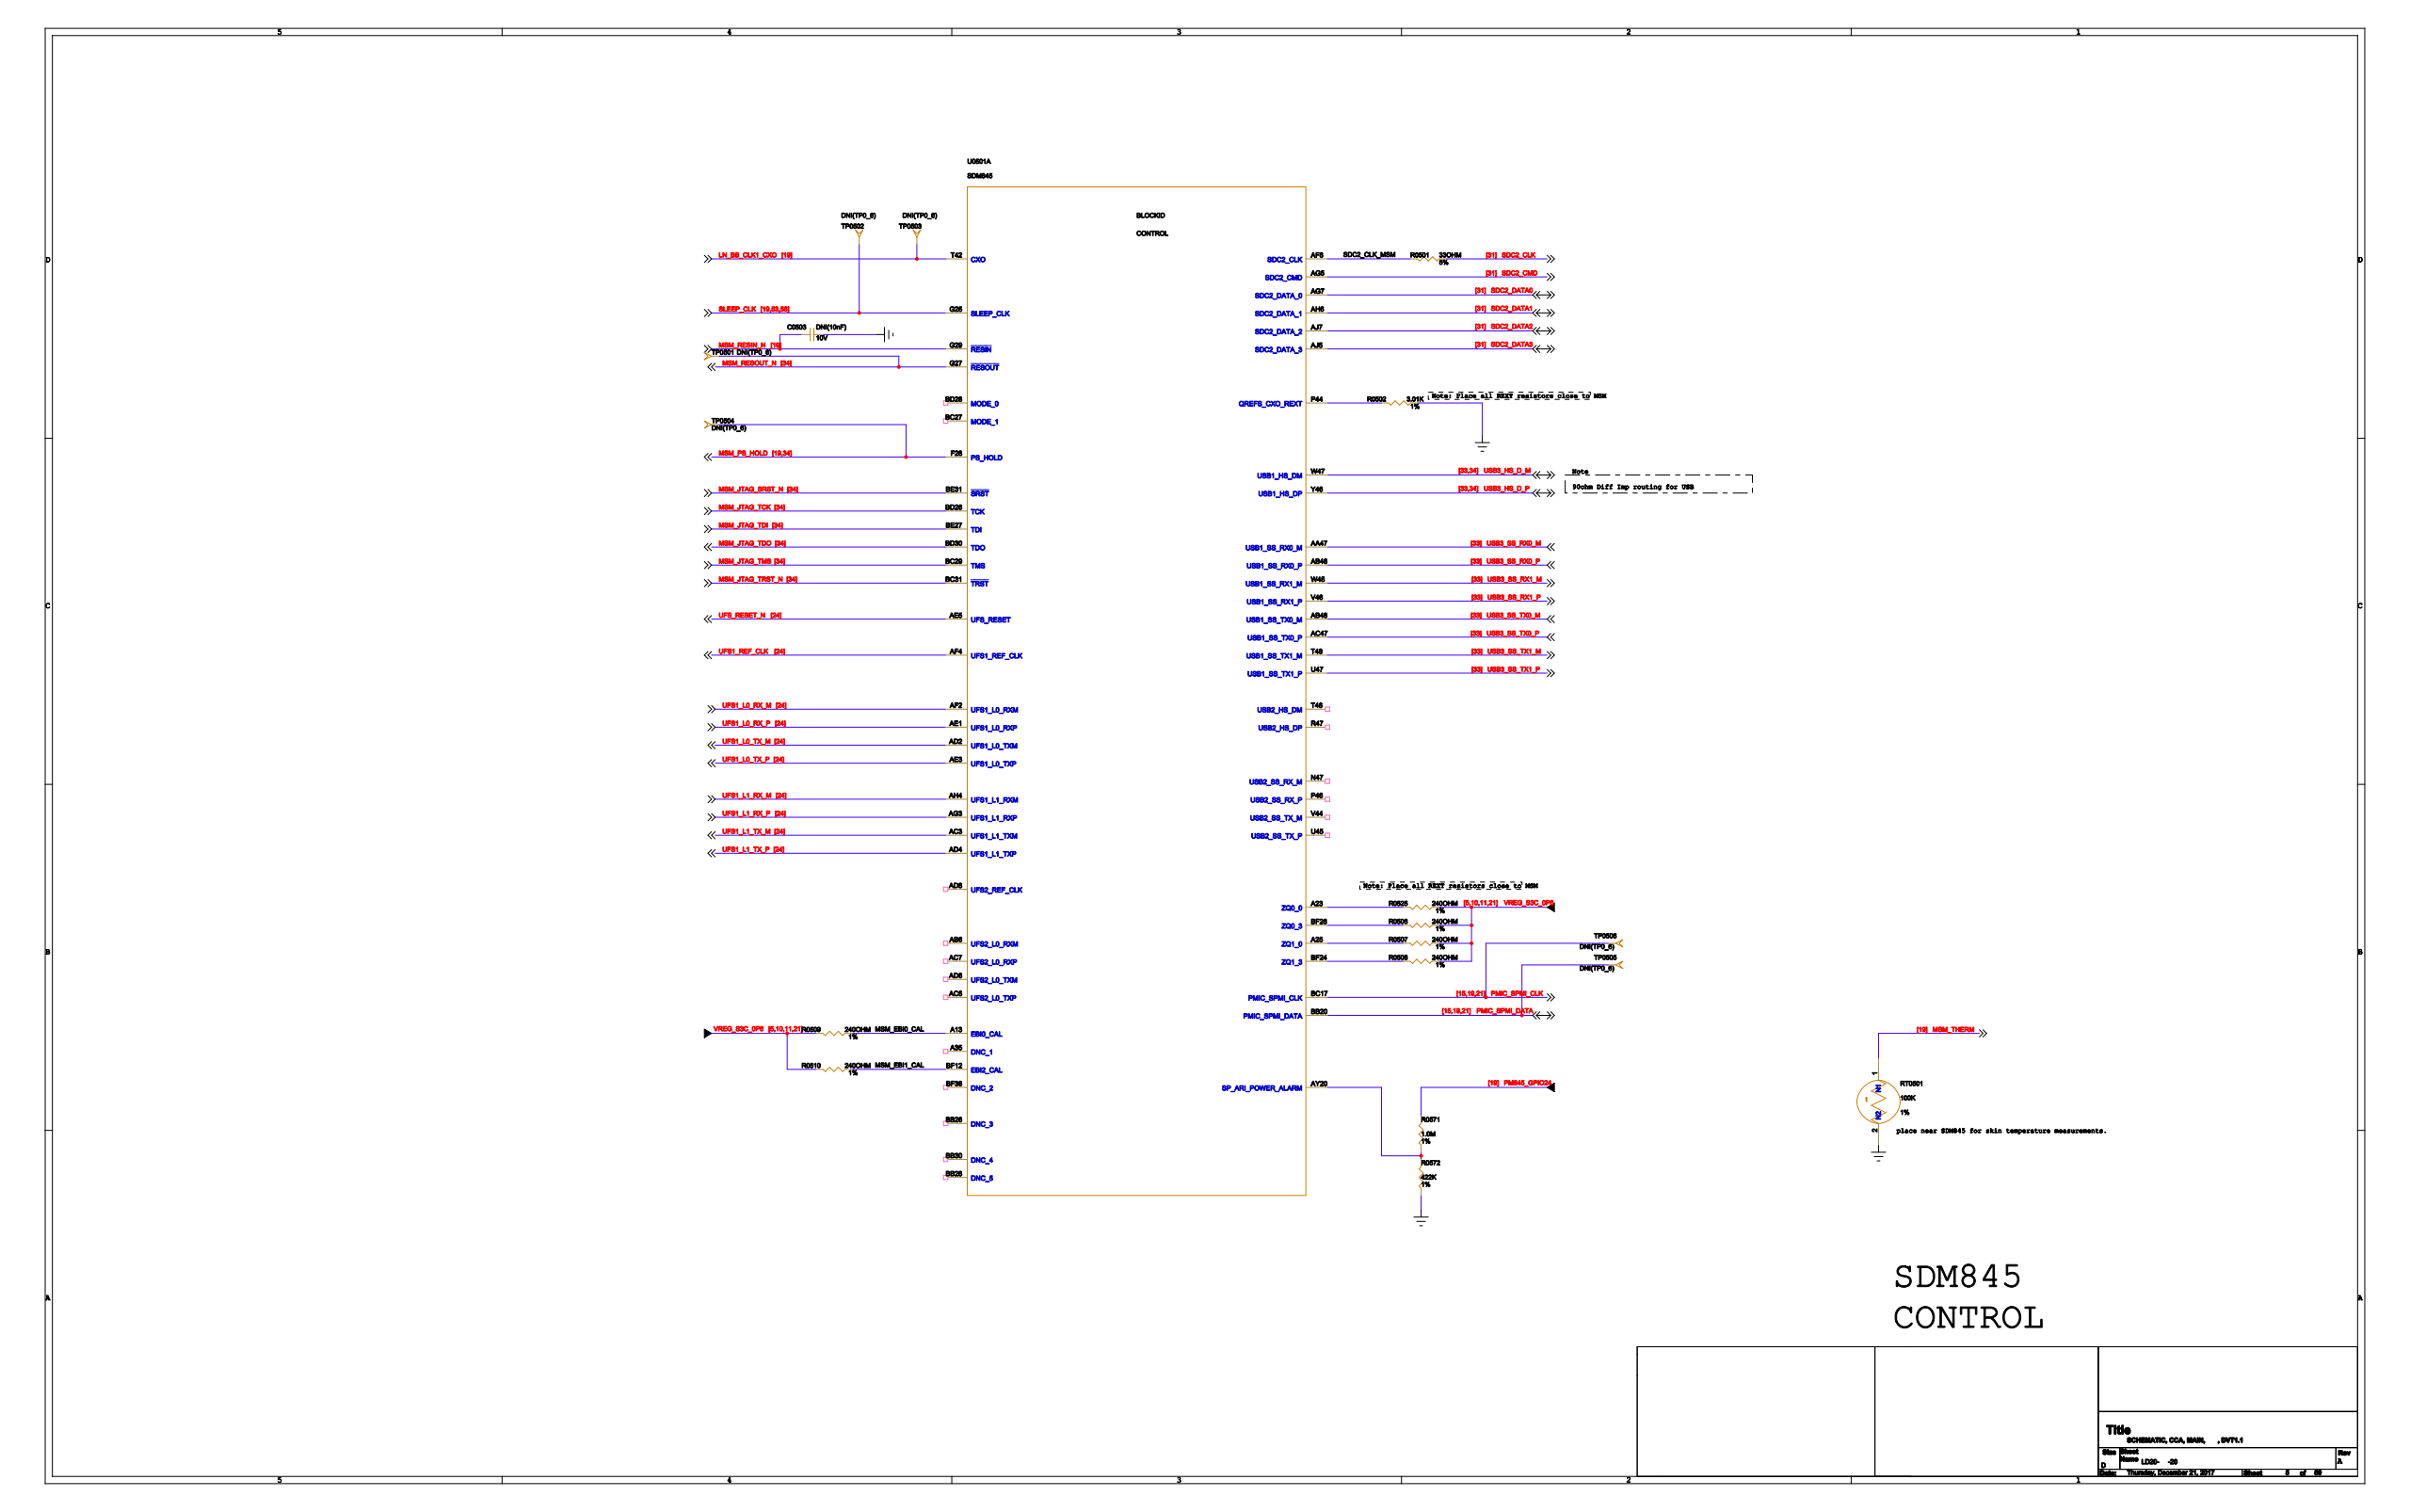Circuit board | Cadence Allegro | 1520 parts | 1149 nets | one sheet of the schematic
Parts on this sheet (reference | value | footprint):
C0503 | DNI(10nF) | 2P0201R_DNI
R0501 | 33OHM | 2P0201R
R0502 | 3.01K | 2P0201R
R0506 | 240OHM | 2P0201R
R0507 | 240OHM | 2P0201R
R0508 | 240OHM | 2P0201R
R0509 | 240OHM | 2P0201R
R0510 | 240OHM | 2P0201R
R0525 | 240OHM | 2P0201R
R0571 | 1.0M | 2P0201R
R0572 | 422K | 2P0201R
RT0501 | 100K | 2P0201R
TP0501 | DNI(TP0_6) | TP-0_6
TP0502 | DNI(TP0_6) | TP-0_6
TP0503 | DNI(TP0_6) | TP-0_6
TP0504 | DNI(TP0_6) | TP-0_6
TP0505 | DNI(TP0_6) | TP-0_6
TP0506 | DNI(TP0_6) | TP-0_6
U0501 | SDM845 | 914PGA490X490B138D45
Nets of these parts (net: part-pin ...):
GND: C0503-2 R0502-2 R0572-2 RT0501-2
SLEEP_CLK: TP0502-1 U0501-G25
VREG_S3C_0P6: R0506-2 R0507-2 R0508-2 R0509-1 R0510-1 R0525-2
MSM_RESIN_N: C0503-1 U0501-G29
USB3_SS_RX0_P: U0501-AB46
USB3_SS_RX0_M: U0501-AA47
USB3_SS_RX1_P: U0501-V46
USB3_SS_RX1_M: U0501-W45
N47040694: R0571-2 R0572-1 U0501-AY20
N47039362: R0502-1 U0501-P44
SDC2_DATA3: U0501-AJ5
SDC2_DATA1: U0501-AH6
SDC2_CMD: U0501-AG5
SDC2_CLK: R0501-2
SDC2_DATA0: U0501-AG7
SDC2_DATA2: U0501-AJ7
USB3_SS_TX0_P: U0501-AC47
USB3_SS_TX0_M: U0501-AB48
USB3_SS_TX1_M: U0501-T48
USB3_SS_TX1_P: U0501-U47
MSM_JTAG_SRST_N: U0501-BE31
MSM_JTAG_TRST_N: U0501-BC31
USB3_HS_D_M: U0501-W47
USB3_HS_D_P: U0501-Y46
MSM_JTAG_TMS: U0501-BC29
MSM_PS_HOLD: TP0504-1 U0501-F28
MSM_RESOUT_N: TP0501-1 U0501-G27
MSM_JTAG_TCK: U0501-BD26
MSM_JTAG_TDO: U0501-BD30
MSM_JTAG_TDI: U0501-BE27
SDC2_CLK_MSM: R0501-1 U0501-AF6
N47039503: R0506-1 U0501-BF26
N47039505: R0507-1 U0501-A25
N47039507: R0508-1 U0501-BF24
MSM_EBI0_CAL: R0509-2 U0501-A13
MSM_EBI1_CAL: R0510-2 U0501-BF12
N47039499: R0525-1 U0501-A23
PM845_GPIO24: R0571-1
MSM_THERM: RT0501-1
PMIC_SPMI_DATA: TP0505-1 U0501-BB20
PMIC_SPMI_CLK: TP0506-1 U0501-BC17
LN_BB_CLK1_CXO: TP0503-1 U0501-T42
UFS1_L0_RX_P: U0501-AE1
UFS1_L0_TX_M: U0501-AD2
UFS1_L0_TX_P: U0501-AE3
UFS1_L0_RX_M: U0501-AF2
UFS1_L1_RX_M: U0501-AH4
UFS1_L1_RX_P: U0501-AG3
UFS1_L1_TX_M: U0501-AC3
UFS1_L1_TX_P: U0501-AD4
UFS1_REF_CLK: U0501-AF4
UFS_RESET_N: U0501-AE5